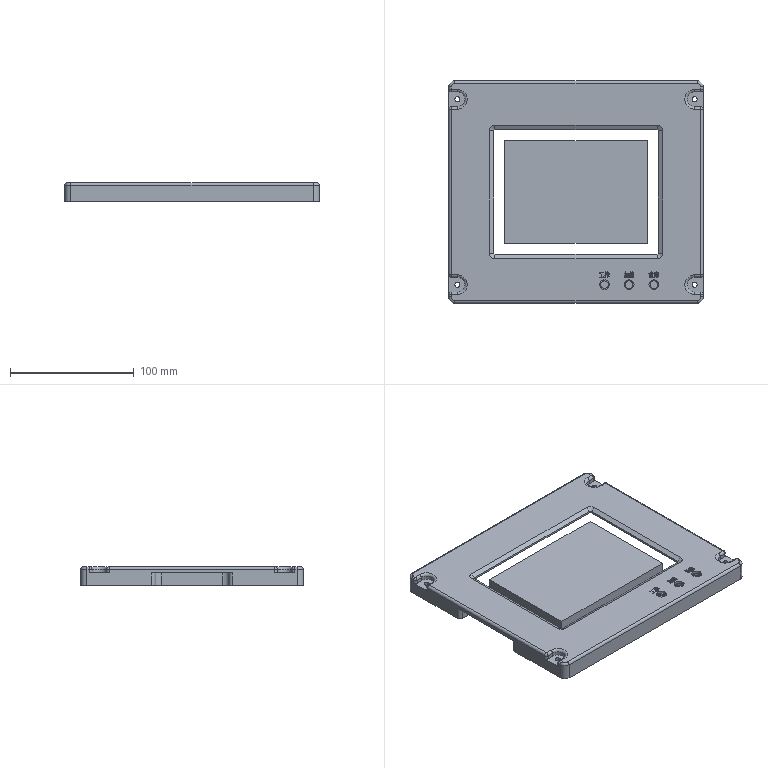Part | 2 solids | 558 faces | box 206 x 180 x 15 mm | volume 246800 mm3 | plane 310 | cylinder 118 | other 98 | cone 12 | torus 8 | sphere 8 | spline 4 | commonest cylinder face diameters 6 x34 4 x28 2.5 x8 4.2 x8 7 x8 10 x8